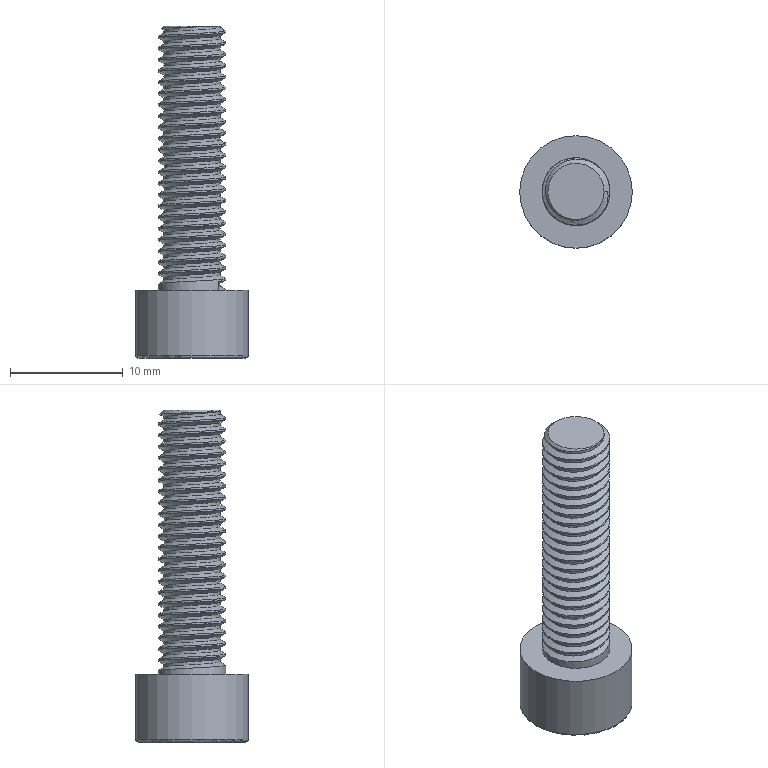Part | STEP file | Tube feed_id1818_x_t | 1 solid | 26 faces | box 10 x 10 x 29.5 mm | volume 955.443 mm3 | plane 12 | cylinder 9 | spline 3 | cone 1 | torus 1 | commonest cylinder face diameters 0.4 x6 5 x1 6 x1 10 x1